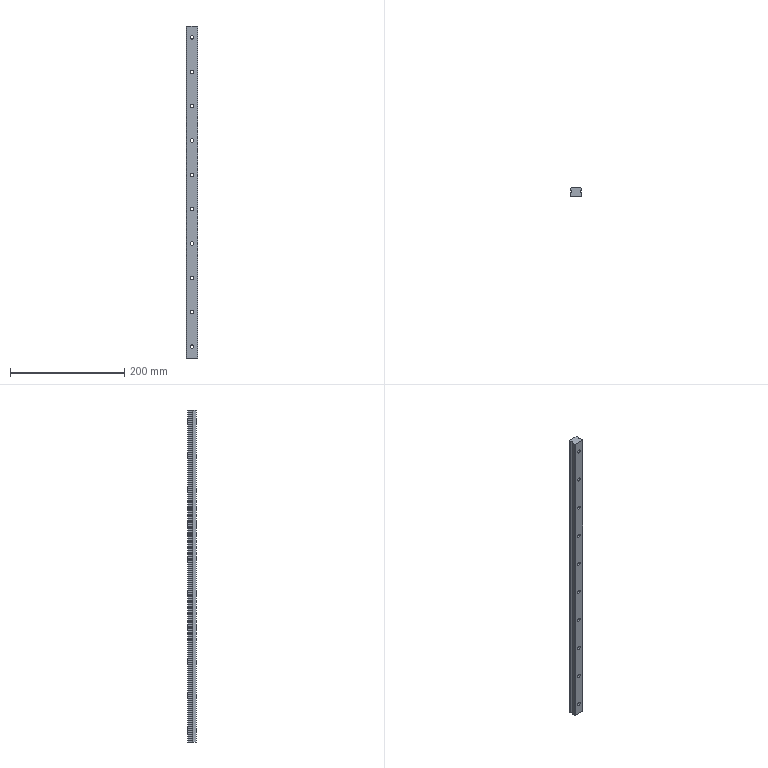Part | NX | features BREP 1 | 1 solid | 67 faces | box 20 x 15.5 x 580 mm | volume 158684 mm3 | cylinder 45 | plane 22 | commonest cylinder face diameters 6 x20 9.5 x20 5 x3 3 x2